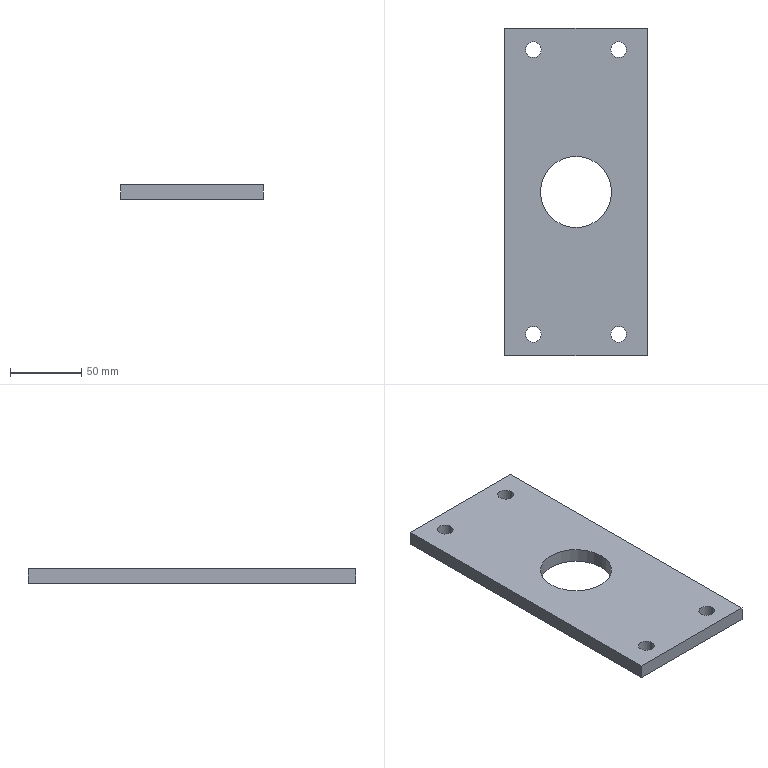Part | SolidWorks | features Extrusion 1 | 1 solid | 16 faces | box 100 x 230 x 10 mm | volume 206564 mm3 | cylinder 10 | plane 6 | commonest cylinder face diameters 11 x8 50 x2
STEP:
#1=CARTESIAN_POINT('',(-35.5,-100.,10.));
#2=VERTEX_POINT('',#1);
#3=CARTESIAN_POINT('',(-24.5,-100.,10.));
#4=VERTEX_POINT('',#3);
#5=CARTESIAN_POINT('',(-30.,-100.,10.));
#6=DIRECTION('',(0.,0.,1.));
#7=DIRECTION('',(1.,0.,0.));
#8=AXIS2_PLACEMENT_3D('',#5,#6,#7);
#9=CIRCLE('',#8,5.5);
#10=EDGE_CURVE('',#2,#4,#9,.T.);
#11=ORIENTED_EDGE('',*,*,#10,.T.);
#12=CARTESIAN_POINT('',(-24.5,-100.,0.));
#13=VERTEX_POINT('',#12);
#14=CARTESIAN_POINT('',(-24.5,-100.,10.));
#15=DIRECTION('',(0.,0.,-1.));
#16=VECTOR('',#15,1000.);
#17=LINE('',#14,#16);
#18=EDGE_CURVE('',#4,#13,#17,.T.);
#19=ORIENTED_EDGE('',*,*,#18,.T.);
#20=CARTESIAN_POINT('',(-35.5,-100.,0.));
#21=VERTEX_POINT('',#20);
#22=CARTESIAN_POINT('',(-30.,-100.,0.));
#23=DIRECTION('',(0.,0.,1.));
#24=DIRECTION('',(1.,0.,0.));
#25=AXIS2_PLACEMENT_3D('',#22,#23,#24);
#26=CIRCLE('',#25,5.5);
#27=EDGE_CURVE('',#21,#13,#26,.T.);
#28=ORIENTED_EDGE('',*,*,#27,.F.);
#29=CARTESIAN_POINT('',(-35.5,-100.,10.));
#30=DIRECTION('',(0.,0.,-1.));
#31=VECTOR('',#30,1000.);
#32=LINE('',#29,#31);
#33=EDGE_CURVE('',#2,#21,#32,.T.);
#34=ORIENTED_EDGE('',*,*,#33,.F.);
#35=EDGE_LOOP('',(#11,#19,#28,#34));
#36=FACE_OUTER_BOUND('',#35,.T.);
#37=CARTESIAN_POINT('',(-30.,-100.,10.));
#38=DIRECTION('',(0.,0.,-1.));
#39=DIRECTION('',(-1.,0.,0.));
#40=AXIS2_PLACEMENT_3D('',#37,#38,#39);
#41=CYLINDRICAL_SURFACE('',#40,5.5);
#42=ADVANCED_FACE('',(#36),#41,.F.);
#43=CARTESIAN_POINT('',(24.5,-100.,10.));
#44=VERTEX_POINT('',#43);
#45=CARTESIAN_POINT('',(35.5,-100.,10.));
#46=VERTEX_POINT('',#45);
#47=CARTESIAN_POINT('',(30.,-100.,10.));
#48=DIRECTION('',(0.,0.,1.));
#49=DIRECTION('',(1.,0.,0.));
#50=AXIS2_PLACEMENT_3D('',#47,#48,#49);
#51=CIRCLE('',#50,5.5);
#52=EDGE_CURVE('',#44,#46,#51,.T.);
#53=ORIENTED_EDGE('',*,*,#52,.T.);
#54=CARTESIAN_POINT('',(35.5,-100.,0.));
#55=VERTEX_POINT('',#54);
#56=CARTESIAN_POINT('',(35.5,-100.,10.));
#57=DIRECTION('',(0.,0.,-1.));
#58=VECTOR('',#57,1000.);
#59=LINE('',#56,#58);
#60=EDGE_CURVE('',#46,#55,#59,.T.);
#61=ORIENTED_EDGE('',*,*,#60,.T.);
#62=CARTESIAN_POINT('',(24.5,-100.,0.));
#63=VERTEX_POINT('',#62);
#64=CARTESIAN_POINT('',(30.,-100.,0.));
#65=DIRECTION('',(0.,0.,1.));
#66=DIRECTION('',(1.,0.,0.));
#67=AXIS2_PLACEMENT_3D('',#64,#65,#66);
#68=CIRCLE('',#67,5.5);
#69=EDGE_CURVE('',#63,#55,#68,.T.);
#70=ORIENTED_EDGE('',*,*,#69,.F.);
#71=CARTESIAN_POINT('',(24.5,-100.,10.));
#72=DIRECTION('',(0.,0.,-1.));
#73=VECTOR('',#72,1000.);
#74=LINE('',#71,#73);
#75=EDGE_CURVE('',#44,#63,#74,.T.);
#76=ORIENTED_EDGE('',*,*,#75,.F.);
#77=EDGE_LOOP('',(#53,#61,#70,#76));
#78=FACE_OUTER_BOUND('',#77,.T.);
#79=CARTESIAN_POINT('',(30.,-100.,10.));
#80=DIRECTION('',(0.,0.,-1.));
#81=DIRECTION('',(-1.,0.,0.));
#82=AXIS2_PLACEMENT_3D('',#79,#80,#81);
#83=CYLINDRICAL_SURFACE('',#82,5.5);
#84=ADVANCED_FACE('',(#78),#83,.F.);
#85=CARTESIAN_POINT('',(24.5,100.,10.));
#86=VERTEX_POINT('',#85);
#87=CARTESIAN_POINT('',(35.5,100.,10.));
#88=VERTEX_POINT('',#87);
#89=CARTESIAN_POINT('',(30.,100.,10.));
#90=DIRECTION('',(0.,0.,1.));
#91=DIRECTION('',(1.,0.,0.));
#92=AXIS2_PLACEMENT_3D('',#89,#90,#91);
#93=CIRCLE('',#92,5.5);
#94=EDGE_CURVE('',#86,#88,#93,.T.);
#95=ORIENTED_EDGE('',*,*,#94,.T.);
#96=CARTESIAN_POINT('',(35.5,100.,0.));
#97=VERTEX_POINT('',#96);
#98=CARTESIAN_POINT('',(35.5,100.,10.));
#99=DIRECTION('',(0.,0.,-1.));
#100=VECTOR('',#99,1000.);
#101=LINE('',#98,#100);
#102=EDGE_CURVE('',#88,#97,#101,.T.);
#103=ORIENTED_EDGE('',*,*,#102,.T.);
#104=CARTESIAN_POINT('',(24.5,100.,0.));
#105=VERTEX_POINT('',#104);
#106=CARTESIAN_POINT('',(30.,100.,0.));
#107=DIRECTION('',(0.,0.,1.));
#108=DIRECTION('',(1.,0.,0.));
#109=AXIS2_PLACEMENT_3D('',#106,#107,#108);
#110=CIRCLE('',#109,5.5);
#111=EDGE_CURVE('',#105,#97,#110,.T.);
#112=ORIENTED_EDGE('',*,*,#111,.F.);
#113=CARTESIAN_POINT('',(24.5,100.,10.));
#114=DIRECTION('',(0.,0.,-1.));
#115=VECTOR('',#114,1000.);
#116=LINE('',#113,#115);
#117=EDGE_CURVE('',#86,#105,#116,.T.);
#118=ORIENTED_EDGE('',*,*,#117,.F.);
#119=EDGE_LOOP('',(#95,#103,#112,#118));
#120=FACE_OUTER_BOUND('',#119,.T.);
#121=CARTESIAN_POINT('',(30.,100.,10.));
#122=DIRECTION('',(0.,0.,-1.));
#123=DIRECTION('',(-1.,0.,0.));
#124=AXIS2_PLACEMENT_3D('',#121,#122,#123);
#125=CYLINDRICAL_SURFACE('',#124,5.5);
#126=ADVANCED_FACE('',(#120),#125,.F.);
#127=CARTESIAN_POINT('',(-35.5,100.,10.));
#128=VERTEX_POINT('',#127);
#129=CARTESIAN_POINT('',(-24.5,100.,10.));
#130=VERTEX_POINT('',#129);
#131=CARTESIAN_POINT('',(-30.,100.,10.));
#132=DIRECTION('',(0.,0.,1.));
#133=DIRECTION('',(1.,0.,0.));
#134=AXIS2_PLACEMENT_3D('',#131,#132,#133);
#135=CIRCLE('',#134,5.5);
#136=EDGE_CURVE('',#128,#130,#135,.T.);
#137=ORIENTED_EDGE('',*,*,#136,.T.);
#138=CARTESIAN_POINT('',(-24.5,100.,0.));
#139=VERTEX_POINT('',#138);
#140=CARTESIAN_POINT('',(-24.5,100.,10.));
#141=DIRECTION('',(0.,0.,-1.));
#142=VECTOR('',#141,1000.);
#143=LINE('',#140,#142);
#144=EDGE_CURVE('',#130,#139,#143,.T.);
#145=ORIENTED_EDGE('',*,*,#144,.T.);
#146=CARTESIAN_POINT('',(-35.5,100.,0.));
#147=VERTEX_POINT('',#146);
#148=CARTESIAN_POINT('',(-30.,100.,0.));
#149=DIRECTION('',(0.,0.,1.));
#150=DIRECTION('',(1.,0.,0.));
#151=AXIS2_PLACEMENT_3D('',#148,#149,#150);
#152=CIRCLE('',#151,5.5);
#153=EDGE_CURVE('',#147,#139,#152,.T.);
#154=ORIENTED_EDGE('',*,*,#153,.F.);
#155=CARTESIAN_POINT('',(-35.5,100.,10.));
#156=DIRECTION('',(0.,0.,-1.));
#157=VECTOR('',#156,1000.);
#158=LINE('',#155,#157);
#159=EDGE_CURVE('',#128,#147,#158,.T.);
#160=ORIENTED_EDGE('',*,*,#159,.F.);
#161=EDGE_LOOP('',(#137,#145,#154,#160));
#162=FACE_OUTER_BOUND('',#161,.T.);
#163=CARTESIAN_POINT('',(-30.,100.,10.));
#164=DIRECTION('',(0.,0.,-1.));
#165=DIRECTION('',(-1.,0.,0.));
#166=AXIS2_PLACEMENT_3D('',#163,#164,#165);
#167=CYLINDRICAL_SURFACE('',#166,5.5);
#168=ADVANCED_FACE('',(#162),#167,.F.);
#169=CARTESIAN_POINT('',(-25.,0.,10.));
#170=VERTEX_POINT('',#169);
#171=CARTESIAN_POINT('',(25.,0.,10.));
#172=VERTEX_POINT('',#171);
#173=CARTESIAN_POINT('',(0.,0.,10.));
#174=DIRECTION('',(0.,0.,1.));
#175=DIRECTION('',(1.,0.,0.));
#176=AXIS2_PLACEMENT_3D('',#173,#174,#175);
#177=CIRCLE('',#176,25.);
#178=EDGE_CURVE('',#170,#172,#177,.T.);
#179=ORIENTED_EDGE('',*,*,#178,.T.);
#180=CARTESIAN_POINT('',(25.,0.,0.));
#181=VERTEX_POINT('',#180);
#182=CARTESIAN_POINT('',(25.,0.,10.));
#183=DIRECTION('',(0.,0.,-1.));
#184=VECTOR('',#183,1000.);
#185=LINE('',#182,#184);
#186=EDGE_CURVE('',#172,#181,#185,.T.);
#187=ORIENTED_EDGE('',*,*,#186,.T.);
#188=CARTESIAN_POINT('',(-25.,0.,0.));
#189=VERTEX_POINT('',#188);
#190=CARTESIAN_POINT('',(0.,0.,0.));
#191=DIRECTION('',(0.,0.,1.));
#192=DIRECTION('',(1.,0.,0.));
#193=AXIS2_PLACEMENT_3D('',#190,#191,#192);
#194=CIRCLE('',#193,25.);
#195=EDGE_CURVE('',#189,#181,#194,.T.);
#196=ORIENTED_EDGE('',*,*,#195,.F.);
#197=CARTESIAN_POINT('',(-25.,0.,10.));
#198=DIRECTION('',(0.,0.,-1.));
#199=VECTOR('',#198,1000.);
#200=LINE('',#197,#199);
#201=EDGE_CURVE('',#170,#189,#200,.T.);
#202=ORIENTED_EDGE('',*,*,#201,.F.);
#203=EDGE_LOOP('',(#179,#187,#196,#202));
#204=FACE_OUTER_BOUND('',#203,.T.);
#205=CARTESIAN_POINT('',(0.,0.,10.));
#206=DIRECTION('',(0.,0.,-1.));
#207=DIRECTION('',(-1.,0.,0.));
#208=AXIS2_PLACEMENT_3D('',#205,#206,#207);
#209=CYLINDRICAL_SURFACE('',#208,25.);
#210=ADVANCED_FACE('',(#204),#209,.F.);
#211=CARTESIAN_POINT('',(50.,-115.,10.));
#212=VERTEX_POINT('',#211);
#213=CARTESIAN_POINT('',(50.,115.,10.));
#214=VERTEX_POINT('',#213);
#215=CARTESIAN_POINT('',(50.,-115.,10.));
#216=DIRECTION('',(0.,1.,0.));
#217=VECTOR('',#216,1000.);
#218=LINE('',#215,#217);
#219=EDGE_CURVE('',#212,#214,#218,.T.);
#220=ORIENTED_EDGE('',*,*,#219,.T.);
#221=CARTESIAN_POINT('',(-50.,115.,10.));
#222=VERTEX_POINT('',#221);
#223=CARTESIAN_POINT('',(-50.,115.,10.));
#224=DIRECTION('',(-1.,0.,0.));
#225=VECTOR('',#224,1000.);
#226=LINE('',#223,#225);
#227=EDGE_CURVE('',#214,#222,#226,.T.);
#228=ORIENTED_EDGE('',*,*,#227,.T.);
#229=CARTESIAN_POINT('',(-50.,-115.,10.));
#230=VERTEX_POINT('',#229);
#231=CARTESIAN_POINT('',(-50.,-115.,10.));
#232=DIRECTION('',(0.,-1.,0.));
#233=VECTOR('',#232,1000.);
#234=LINE('',#231,#233);
#235=EDGE_CURVE('',#222,#230,#234,.T.);
#236=ORIENTED_EDGE('',*,*,#235,.T.);
#237=CARTESIAN_POINT('',(-50.,-115.,10.));
#238=DIRECTION('',(1.,0.,0.));
#239=VECTOR('',#238,1000.);
#240=LINE('',#237,#239);
#241=EDGE_CURVE('',#230,#212,#240,.T.);
#242=ORIENTED_EDGE('',*,*,#241,.T.);
#243=EDGE_LOOP('',(#220,#228,#236,#242));
#244=FACE_OUTER_BOUND('',#243,.T.);
#245=ORIENTED_EDGE('',*,*,#178,.F.);
#246=CARTESIAN_POINT('',(0.,0.,10.));
#247=DIRECTION('',(0.,0.,1.));
#248=DIRECTION('',(1.,0.,0.));
#249=AXIS2_PLACEMENT_3D('',#246,#247,#248);
#250=CIRCLE('',#249,25.);
#251=EDGE_CURVE('',#172,#170,#250,.T.);
#252=ORIENTED_EDGE('',*,*,#251,.F.);
#253=EDGE_LOOP('',(#245,#252));
#254=FACE_BOUND('',#253,.T.);
#255=ORIENTED_EDGE('',*,*,#136,.F.);
#256=CARTESIAN_POINT('',(-30.,100.,10.));
#257=DIRECTION('',(0.,0.,1.));
#258=DIRECTION('',(1.,0.,0.));
#259=AXIS2_PLACEMENT_3D('',#256,#257,#258);
#260=CIRCLE('',#259,5.5);
#261=EDGE_CURVE('',#130,#128,#260,.T.);
#262=ORIENTED_EDGE('',*,*,#261,.F.);
#263=EDGE_LOOP('',(#255,#262));
#264=FACE_BOUND('',#263,.T.);
#265=ORIENTED_EDGE('',*,*,#94,.F.);
#266=CARTESIAN_POINT('',(30.,100.,10.));
#267=DIRECTION('',(0.,0.,1.));
#268=DIRECTION('',(1.,0.,0.));
#269=AXIS2_PLACEMENT_3D('',#266,#267,#268);
#270=CIRCLE('',#269,5.5);
#271=EDGE_CURVE('',#88,#86,#270,.T.);
#272=ORIENTED_EDGE('',*,*,#271,.F.);
#273=EDGE_LOOP('',(#265,#272));
#274=FACE_BOUND('',#273,.T.);
#275=ORIENTED_EDGE('',*,*,#52,.F.);
#276=CARTESIAN_POINT('',(30.,-100.,10.));
#277=DIRECTION('',(0.,0.,1.));
#278=DIRECTION('',(1.,0.,0.));
#279=AXIS2_PLACEMENT_3D('',#276,#277,#278);
#280=CIRCLE('',#279,5.5);
#281=EDGE_CURVE('',#46,#44,#280,.T.);
#282=ORIENTED_EDGE('',*,*,#281,.F.);
#283=EDGE_LOOP('',(#275,#282));
#284=FACE_BOUND('',#283,.T.);
#285=ORIENTED_EDGE('',*,*,#10,.F.);
#286=CARTESIAN_POINT('',(-30.,-100.,10.));
#287=DIRECTION('',(0.,0.,1.));
#288=DIRECTION('',(1.,0.,0.));
#289=AXIS2_PLACEMENT_3D('',#286,#287,#288);
#290=CIRCLE('',#289,5.5);
#291=EDGE_CURVE('',#4,#2,#290,.T.);
#292=ORIENTED_EDGE('',*,*,#291,.F.);
#293=EDGE_LOOP('',(#285,#292));
#294=FACE_BOUND('',#293,.T.);
#295=CARTESIAN_POINT('',(0.,0.,10.));
#296=DIRECTION('',(0.,0.,-1.));
#297=DIRECTION('',(-1.,0.,0.));
#298=AXIS2_PLACEMENT_3D('',#295,#296,#297);
#299=PLANE('',#298);
#300=ADVANCED_FACE('',(#244,#254,#264,#274,#284,#294),#299,.F.);
#301=ORIENTED_EDGE('',*,*,#69,.T.);
#302=CARTESIAN_POINT('',(30.,-100.,0.));
#303=DIRECTION('',(0.,0.,1.));
#304=DIRECTION('',(1.,0.,0.));
#305=AXIS2_PLACEMENT_3D('',#302,#303,#304);
#306=CIRCLE('',#305,5.5);
#307=EDGE_CURVE('',#55,#63,#306,.T.);
#308=ORIENTED_EDGE('',*,*,#307,.T.);
#309=EDGE_LOOP('',(#301,#308));
#310=FACE_BOUND('',#309,.T.);
#311=ORIENTED_EDGE('',*,*,#153,.T.);
#312=CARTESIAN_POINT('',(-30.,100.,0.));
#313=DIRECTION('',(0.,0.,1.));
#314=DIRECTION('',(1.,0.,0.));
#315=AXIS2_PLACEMENT_3D('',#312,#313,#314);
#316=CIRCLE('',#315,5.5);
#317=EDGE_CURVE('',#139,#147,#316,.T.);
#318=ORIENTED_EDGE('',*,*,#317,.T.);
#319=EDGE_LOOP('',(#311,#318));
#320=FACE_BOUND('',#319,.T.);
#321=CARTESIAN_POINT('',(50.,-115.,0.));
#322=VERTEX_POINT('',#321);
#323=CARTESIAN_POINT('',(50.,115.,0.));
#324=VERTEX_POINT('',#323);
#325=CARTESIAN_POINT('',(50.,-115.,0.));
#326=DIRECTION('',(0.,1.,0.));
#327=VECTOR('',#326,1000.);
#328=LINE('',#325,#327);
#329=EDGE_CURVE('',#322,#324,#328,.T.);
#330=ORIENTED_EDGE('',*,*,#329,.F.);
#331=CARTESIAN_POINT('',(-50.,-115.,0.));
#332=VERTEX_POINT('',#331);
#333=CARTESIAN_POINT('',(-50.,-115.,0.));
#334=DIRECTION('',(1.,0.,0.));
#335=VECTOR('',#334,1000.);
#336=LINE('',#333,#335);
#337=EDGE_CURVE('',#332,#322,#336,.T.);
#338=ORIENTED_EDGE('',*,*,#337,.F.);
#339=CARTESIAN_POINT('',(-50.,115.,0.));
#340=VERTEX_POINT('',#339);
#341=CARTESIAN_POINT('',(-50.,-115.,0.));
#342=DIRECTION('',(0.,-1.,0.));
#343=VECTOR('',#342,1000.);
#344=LINE('',#341,#343);
#345=EDGE_CURVE('',#340,#332,#344,.T.);
#346=ORIENTED_EDGE('',*,*,#345,.F.);
#347=CARTESIAN_POINT('',(-50.,115.,0.));
#348=DIRECTION('',(-1.,0.,0.));
#349=VECTOR('',#348,1000.);
#350=LINE('',#347,#349);
#351=EDGE_CURVE('',#324,#340,#350,.T.);
#352=ORIENTED_EDGE('',*,*,#351,.F.);
#353=EDGE_LOOP('',(#330,#338,#346,#352));
#354=FACE_OUTER_BOUND('',#353,.T.);
#355=ORIENTED_EDGE('',*,*,#195,.T.);
#356=CARTESIAN_POINT('',(0.,0.,0.));
#357=DIRECTION('',(0.,0.,1.));
#358=DIRECTION('',(1.,0.,0.));
#359=AXIS2_PLACEMENT_3D('',#356,#357,#358);
#360=CIRCLE('',#359,25.);
#361=EDGE_CURVE('',#181,#189,#360,.T.);
#362=ORIENTED_EDGE('',*,*,#361,.T.);
#363=EDGE_LOOP('',(#355,#362));
#364=FACE_BOUND('',#363,.T.);
#365=ORIENTED_EDGE('',*,*,#111,.T.);
#366=CARTESIAN_POINT('',(30.,100.,0.));
#367=DIRECTION('',(0.,0.,1.));
#368=DIRECTION('',(1.,0.,0.));
#369=AXIS2_PLACEMENT_3D('',#366,#367,#368);
#370=CIRCLE('',#369,5.5);
#371=EDGE_CURVE('',#97,#105,#370,.T.);
#372=ORIENTED_EDGE('',*,*,#371,.T.);
#373=EDGE_LOOP('',(#365,#372));
#374=FACE_BOUND('',#373,.T.);
#375=ORIENTED_EDGE('',*,*,#27,.T.);
#376=CARTESIAN_POINT('',(-30.,-100.,0.));
#377=DIRECTION('',(0.,0.,1.));
#378=DIRECTION('',(1.,0.,0.));
#379=AXIS2_PLACEMENT_3D('',#376,#377,#378);
#380=CIRCLE('',#379,5.5);
#381=EDGE_CURVE('',#13,#21,#380,.T.);
#382=ORIENTED_EDGE('',*,*,#381,.T.);
#383=EDGE_LOOP('',(#375,#382));
#384=FACE_BOUND('',#383,.T.);
#385=CARTESIAN_POINT('',(0.,0.,0.));
#386=DIRECTION('',(0.,0.,-1.));
#387=DIRECTION('',(-1.,0.,0.));
#388=AXIS2_PLACEMENT_3D('',#385,#386,#387);
#389=PLANE('',#388);
#390=ADVANCED_FACE('',(#310,#320,#354,#364,#374,#384),#389,.T.);
#391=ORIENTED_EDGE('',*,*,#329,.T.);
#392=CARTESIAN_POINT('',(50.,115.,10.));
#393=DIRECTION('',(0.,0.,-1.));
#394=VECTOR('',#393,1000.);
#395=LINE('',#392,#394);
#396=EDGE_CURVE('',#214,#324,#395,.T.);
#397=ORIENTED_EDGE('',*,*,#396,.F.);
#398=ORIENTED_EDGE('',*,*,#219,.F.);
#399=CARTESIAN_POINT('',(50.,-115.,10.));
#400=DIRECTION('',(0.,0.,-1.));
#401=VECTOR('',#400,1000.);
#402=LINE('',#399,#401);
#403=EDGE_CURVE('',#212,#322,#402,.T.);
#404=ORIENTED_EDGE('',*,*,#403,.T.);
#405=EDGE_LOOP('',(#391,#397,#398,#404));
#406=FACE_OUTER_BOUND('',#405,.T.);
#407=CARTESIAN_POINT('',(50.,-115.,10.));
#408=DIRECTION('',(-1.,0.,0.));
#409=DIRECTION('',(0.,0.,1.));
#410=AXIS2_PLACEMENT_3D('',#407,#408,#409);
#411=PLANE('',#410);
#412=ADVANCED_FACE('',(#406),#411,.F.);
#413=ORIENTED_EDGE('',*,*,#351,.T.);
#414=CARTESIAN_POINT('',(-50.,115.,10.));
#415=DIRECTION('',(0.,0.,-1.));
#416=VECTOR('',#415,1000.);
#417=LINE('',#414,#416);
#418=EDGE_CURVE('',#222,#340,#417,.T.);
#419=ORIENTED_EDGE('',*,*,#418,.F.);
#420=ORIENTED_EDGE('',*,*,#227,.F.);
#421=ORIENTED_EDGE('',*,*,#396,.T.);
#422=EDGE_LOOP('',(#413,#419,#420,#421));
#423=FACE_OUTER_BOUND('',#422,.T.);
#424=CARTESIAN_POINT('',(-50.,115.,10.));
#425=DIRECTION('',(0.,-1.,0.));
#426=DIRECTION('',(0.,0.,-1.));
#427=AXIS2_PLACEMENT_3D('',#424,#425,#426);
#428=PLANE('',#427);
#429=ADVANCED_FACE('',(#423),#428,.F.);
#430=ORIENTED_EDGE('',*,*,#345,.T.);
#431=CARTESIAN_POINT('',(-50.,-115.,10.));
#432=DIRECTION('',(0.,0.,-1.));
#433=VECTOR('',#432,1000.);
#434=LINE('',#431,#433);
#435=EDGE_CURVE('',#230,#332,#434,.T.);
#436=ORIENTED_EDGE('',*,*,#435,.F.);
#437=ORIENTED_EDGE('',*,*,#235,.F.);
#438=ORIENTED_EDGE('',*,*,#418,.T.);
#439=EDGE_LOOP('',(#430,#436,#437,#438));
#440=FACE_OUTER_BOUND('',#439,.T.);
#441=CARTESIAN_POINT('',(-50.,-115.,10.));
#442=DIRECTION('',(1.,0.,0.));
#443=DIRECTION('',(0.,0.,-1.));
#444=AXIS2_PLACEMENT_3D('',#441,#442,#443);
#445=PLANE('',#444);
#446=ADVANCED_FACE('',(#440),#445,.F.);
#447=ORIENTED_EDGE('',*,*,#337,.T.);
#448=ORIENTED_EDGE('',*,*,#403,.F.);
#449=ORIENTED_EDGE('',*,*,#241,.F.);
#450=ORIENTED_EDGE('',*,*,#435,.T.);
#451=EDGE_LOOP('',(#447,#448,#449,#450));
#452=FACE_OUTER_BOUND('',#451,.T.);
#453=CARTESIAN_POINT('',(-50.,-115.,10.));
#454=DIRECTION('',(0.,1.,0.));
#455=DIRECTION('',(0.,0.,1.));
#456=AXIS2_PLACEMENT_3D('',#453,#454,#455);
#457=PLANE('',#456);
#458=ADVANCED_FACE('',(#452),#457,.F.);
#459=ORIENTED_EDGE('',*,*,#186,.F.);
#460=ORIENTED_EDGE('',*,*,#251,.T.);
#461=ORIENTED_EDGE('',*,*,#201,.T.);
#462=ORIENTED_EDGE('',*,*,#361,.F.);
#463=EDGE_LOOP('',(#459,#460,#461,#462));
#464=FACE_OUTER_BOUND('',#463,.T.);
#465=CARTESIAN_POINT('',(0.,0.,10.));
#466=DIRECTION('',(0.,0.,-1.));
#467=DIRECTION('',(-1.,0.,0.));
#468=AXIS2_PLACEMENT_3D('',#465,#466,#467);
#469=CYLINDRICAL_SURFACE('',#468,25.);
#470=ADVANCED_FACE('',(#464),#469,.F.);
#471=ORIENTED_EDGE('',*,*,#144,.F.);
#472=ORIENTED_EDGE('',*,*,#261,.T.);
#473=ORIENTED_EDGE('',*,*,#159,.T.);
#474=ORIENTED_EDGE('',*,*,#317,.F.);
#475=EDGE_LOOP('',(#471,#472,#473,#474));
#476=FACE_OUTER_BOUND('',#475,.T.);
#477=CARTESIAN_POINT('',(-30.,100.,10.));
#478=DIRECTION('',(0.,0.,-1.));
#479=DIRECTION('',(-1.,0.,0.));
#480=AXIS2_PLACEMENT_3D('',#477,#478,#479);
#481=CYLINDRICAL_SURFACE('',#480,5.5);
#482=ADVANCED_FACE('',(#476),#481,.F.);
#483=ORIENTED_EDGE('',*,*,#102,.F.);
#484=ORIENTED_EDGE('',*,*,#271,.T.);
#485=ORIENTED_EDGE('',*,*,#117,.T.);
#486=ORIENTED_EDGE('',*,*,#371,.F.);
#487=EDGE_LOOP('',(#483,#484,#485,#486));
#488=FACE_OUTER_BOUND('',#487,.T.);
#489=CARTESIAN_POINT('',(30.,100.,10.));
#490=DIRECTION('',(0.,0.,-1.));
#491=DIRECTION('',(-1.,0.,0.));
#492=AXIS2_PLACEMENT_3D('',#489,#490,#491);
#493=CYLINDRICAL_SURFACE('',#492,5.5);
#494=ADVANCED_FACE('',(#488),#493,.F.);
#495=ORIENTED_EDGE('',*,*,#60,.F.);
#496=ORIENTED_EDGE('',*,*,#281,.T.);
#497=ORIENTED_EDGE('',*,*,#75,.T.);
#498=ORIENTED_EDGE('',*,*,#307,.F.);
#499=EDGE_LOOP('',(#495,#496,#497,#498));
#500=FACE_OUTER_BOUND('',#499,.T.);
#501=CARTESIAN_POINT('',(30.,-100.,10.));
#502=DIRECTION('',(0.,0.,-1.));
#503=DIRECTION('',(-1.,0.,0.));
#504=AXIS2_PLACEMENT_3D('',#501,#502,#503);
#505=CYLINDRICAL_SURFACE('',#504,5.5);
#506=ADVANCED_FACE('',(#500),#505,.F.);
#507=ORIENTED_EDGE('',*,*,#18,.F.);
#508=ORIENTED_EDGE('',*,*,#291,.T.);
#509=ORIENTED_EDGE('',*,*,#33,.T.);
#510=ORIENTED_EDGE('',*,*,#381,.F.);
#511=EDGE_LOOP('',(#507,#508,#509,#510));
#512=FACE_OUTER_BOUND('',#511,.T.);
#513=CARTESIAN_POINT('',(-30.,-100.,10.));
#514=DIRECTION('',(0.,0.,-1.));
#515=DIRECTION('',(-1.,0.,0.));
#516=AXIS2_PLACEMENT_3D('',#513,#514,#515);
#517=CYLINDRICAL_SURFACE('',#516,5.5);
#518=ADVANCED_FACE('',(#512),#517,.F.);
#519=CLOSED_SHELL('',(#42,#84,#126,#168,#210,#300,#390,#412,#429,#446,#458,#470,#482,#494,#506,#518));
#520=MANIFOLD_SOLID_BREP('',#519);
#521=CARTESIAN_POINT('',(0.,0.,0.));
#522=DIRECTION('',(0.,0.,1.));
#523=DIRECTION('',(1.,0.,0.));
#524=AXIS2_PLACEMENT_3D('',#521,#522,#523);
#525=(LENGTH_UNIT()NAMED_UNIT(*)SI_UNIT(.MILLI.,.METRE.));
#526=UNCERTAINTY_MEASURE_WITH_UNIT(LENGTH_MEASURE(0.00001),#525,'','');
#527=(NAMED_UNIT(*)PLANE_ANGLE_UNIT()SI_UNIT($,.RADIAN.));
#528=(NAMED_UNIT(*)SI_UNIT($,.STERADIAN.)SOLID_ANGLE_UNIT());
#529=(GEOMETRIC_REPRESENTATION_CONTEXT(3)GLOBAL_UNCERTAINTY_ASSIGNED_CONTEXT((#526))GLOBAL_UNIT_ASSIGNED_CONTEXT((#525,#527,#528))REPRESENTATION_CONTEXT('',''));
#530=ADVANCED_BREP_SHAPE_REPRESENTATION('',(#520,#524),#529);